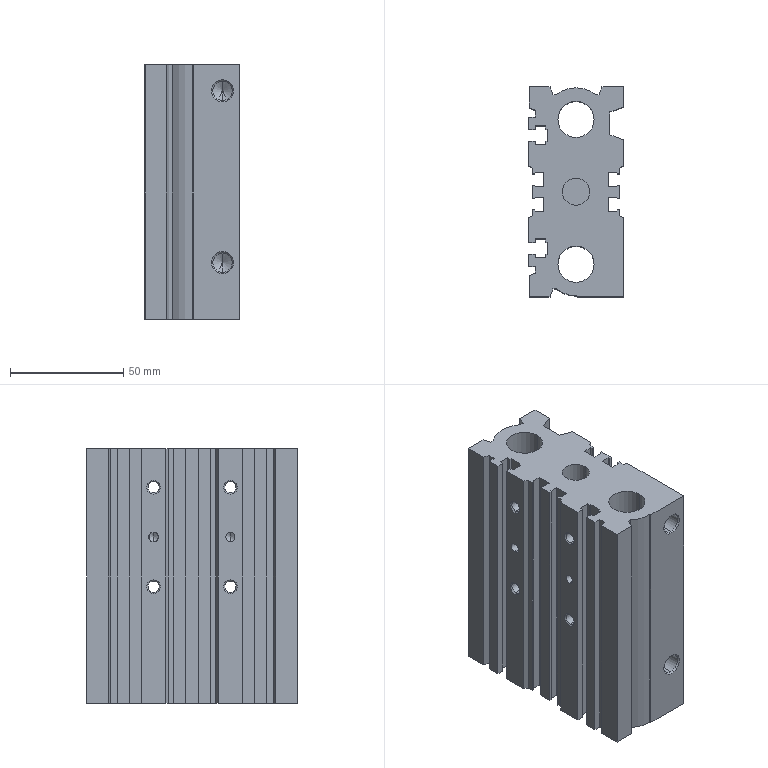Part | SolidWorks | features BaseBody 1 | 1 solid | 215 faces | box 42 x 93 x 112.5 mm | volume 290888 mm3 | plane 113 | cylinder 62 | cone 40 | commonest cylinder face diameters 4.917 x16 4 x12 5.4 x8 8.566 x8 9.5 x8 16 x4